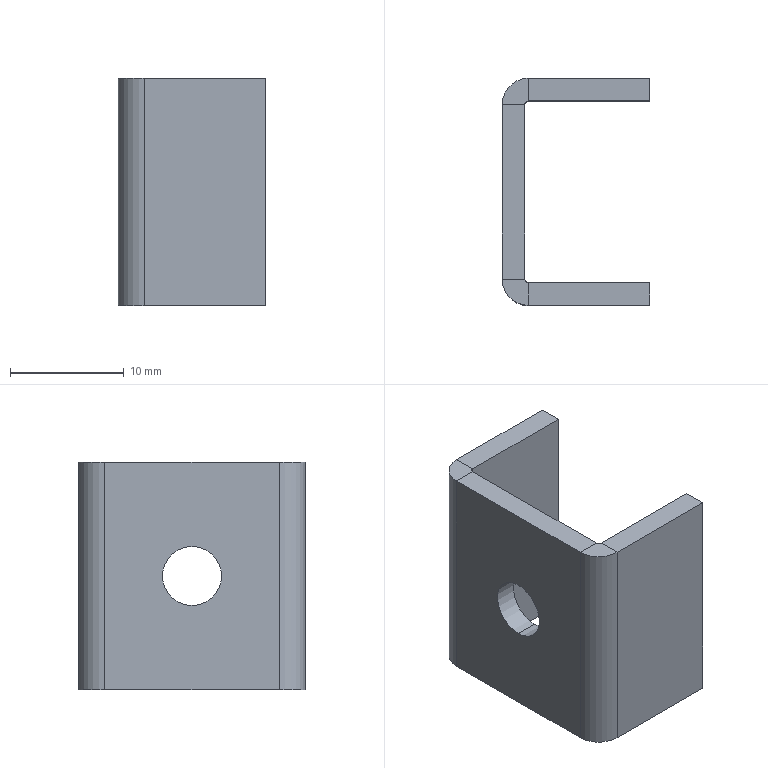Part | SolidWorks | features Cut 1, FlatPattern 1, SMBaseFlange 1, SheetMetal 1 | 1 solid | 24 faces | box 13 x 20 x 20 mm | volume 1593 mm3 | plane 18 | cylinder 6 | commonest cylinder face diameters 0.6 x2 4.6 x2 5.2 x2
STEP:
#1=CARTESIAN_POINT('',(2.,10.,7.4));
#2=VERTEX_POINT('',#1);
#3=CARTESIAN_POINT('',(2.,10.,12.6));
#4=VERTEX_POINT('',#3);
#5=CARTESIAN_POINT('',(2.,10.,10.));
#6=DIRECTION('',(-1.,0.,0.));
#7=DIRECTION('',(0.,0.,1.));
#8=AXIS2_PLACEMENT_3D('',#5,#6,#7);
#9=CIRCLE('',#8,2.6);
#10=EDGE_CURVE('',#2,#4,#9,.T.);
#11=ORIENTED_EDGE('',*,*,#10,.F.);
#12=CARTESIAN_POINT('',(0.,10.,7.4));
#13=VERTEX_POINT('',#12);
#14=CARTESIAN_POINT('',(2.,10.,7.4));
#15=DIRECTION('',(-1.,0.,0.));
#16=VECTOR('',#15,1000.);
#17=LINE('',#14,#16);
#18=EDGE_CURVE('',#2,#13,#17,.T.);
#19=ORIENTED_EDGE('',*,*,#18,.T.);
#20=CARTESIAN_POINT('',(0.,10.,12.6));
#21=VERTEX_POINT('',#20);
#22=CARTESIAN_POINT('',(0.,10.,10.));
#23=DIRECTION('',(-1.,0.,0.));
#24=DIRECTION('',(0.,0.,1.));
#25=AXIS2_PLACEMENT_3D('',#22,#23,#24);
#26=CIRCLE('',#25,2.6);
#27=EDGE_CURVE('',#13,#21,#26,.T.);
#28=ORIENTED_EDGE('',*,*,#27,.T.);
#29=CARTESIAN_POINT('',(2.,10.,12.6));
#30=DIRECTION('',(-1.,0.,0.));
#31=VECTOR('',#30,1000.);
#32=LINE('',#29,#31);
#33=EDGE_CURVE('',#4,#21,#32,.T.);
#34=ORIENTED_EDGE('',*,*,#33,.F.);
#35=EDGE_LOOP('',(#11,#19,#28,#34));
#36=FACE_OUTER_BOUND('',#35,.T.);
#37=CARTESIAN_POINT('',(2.,10.,10.));
#38=DIRECTION('',(-1.,0.,0.));
#39=DIRECTION('',(0.,0.,1.));
#40=AXIS2_PLACEMENT_3D('',#37,#38,#39);
#41=CYLINDRICAL_SURFACE('',#40,2.6);
#42=ADVANCED_FACE('',(#36),#41,.F.);
#43=CARTESIAN_POINT('',(0.,2.3,20.));
#44=VERTEX_POINT('',#43);
#45=CARTESIAN_POINT('',(2.,2.3,20.));
#46=VERTEX_POINT('',#45);
#47=CARTESIAN_POINT('',(0.,2.3,20.));
#48=DIRECTION('',(1.,0.,0.));
#49=VECTOR('',#48,1000.);
#50=LINE('',#47,#49);
#51=EDGE_CURVE('',#44,#46,#50,.T.);
#52=ORIENTED_EDGE('',*,*,#51,.F.);
#53=CARTESIAN_POINT('',(2.3,0.,20.));
#54=VERTEX_POINT('',#53);
#55=CARTESIAN_POINT('',(2.3,2.3,20.));
#56=DIRECTION('',(0.,0.,-1.));
#57=DIRECTION('',(1.,0.,0.));
#58=AXIS2_PLACEMENT_3D('',#55,#56,#57);
#59=CIRCLE('',#58,2.3);
#60=EDGE_CURVE('',#54,#44,#59,.T.);
#61=ORIENTED_EDGE('',*,*,#60,.F.);
#62=CARTESIAN_POINT('',(2.3,2.,20.));
#63=VERTEX_POINT('',#62);
#64=CARTESIAN_POINT('',(2.3,2.,20.));
#65=DIRECTION('',(0.,-1.,0.));
#66=VECTOR('',#65,1000.);
#67=LINE('',#64,#66);
#68=EDGE_CURVE('',#63,#54,#67,.T.);
#69=ORIENTED_EDGE('',*,*,#68,.F.);
#70=CARTESIAN_POINT('',(2.3,2.3,20.));
#71=DIRECTION('',(0.,0.,-1.));
#72=DIRECTION('',(1.,0.,0.));
#73=AXIS2_PLACEMENT_3D('',#70,#71,#72);
#74=CIRCLE('',#73,0.3);
#75=EDGE_CURVE('',#63,#46,#74,.T.);
#76=ORIENTED_EDGE('',*,*,#75,.T.);
#77=EDGE_LOOP('',(#52,#61,#69,#76));
#78=FACE_OUTER_BOUND('',#77,.T.);
#79=CARTESIAN_POINT('',(0.,2.3,20.));
#80=DIRECTION('',(0.,0.,1.));
#81=DIRECTION('',(1.,0.,0.));
#82=AXIS2_PLACEMENT_3D('',#79,#80,#81);
#83=PLANE('',#82);
#84=ADVANCED_FACE('',(#78),#83,.T.);
#85=CARTESIAN_POINT('',(0.,17.7,20.));
#86=VERTEX_POINT('',#85);
#87=CARTESIAN_POINT('',(0.,0.,20.));
#88=DIRECTION('',(0.,1.,0.));
#89=VECTOR('',#88,1000.);
#90=LINE('',#87,#89);
#91=EDGE_CURVE('',#44,#86,#90,.T.);
#92=ORIENTED_EDGE('',*,*,#91,.F.);
#93=ORIENTED_EDGE('',*,*,#51,.T.);
#94=CARTESIAN_POINT('',(2.,17.7,20.));
#95=VERTEX_POINT('',#94);
#96=CARTESIAN_POINT('',(2.,0.,20.));
#97=DIRECTION('',(0.,1.,0.));
#98=VECTOR('',#97,1000.);
#99=LINE('',#96,#98);
#100=EDGE_CURVE('',#46,#95,#99,.T.);
#101=ORIENTED_EDGE('',*,*,#100,.T.);
#102=CARTESIAN_POINT('',(2.,17.7,20.));
#103=DIRECTION('',(-1.,0.,0.));
#104=VECTOR('',#103,1000.);
#105=LINE('',#102,#104);
#106=EDGE_CURVE('',#95,#86,#105,.T.);
#107=ORIENTED_EDGE('',*,*,#106,.T.);
#108=EDGE_LOOP('',(#92,#93,#101,#107));
#109=FACE_OUTER_BOUND('',#108,.T.);
#110=CARTESIAN_POINT('',(2.3,2.,20.));
#111=DIRECTION('',(0.,0.,1.));
#112=DIRECTION('',(1.,0.,0.));
#113=AXIS2_PLACEMENT_3D('',#110,#111,#112);
#114=PLANE('',#113);
#115=ADVANCED_FACE('',(#109),#114,.T.);
#116=CARTESIAN_POINT('',(2.3,0.,0.));
#117=VERTEX_POINT('',#116);
#118=CARTESIAN_POINT('',(2.3,2.,0.));
#119=VERTEX_POINT('',#118);
#120=CARTESIAN_POINT('',(2.3,0.,0.));
#121=DIRECTION('',(0.,1.,0.));
#122=VECTOR('',#121,1000.);
#123=LINE('',#120,#122);
#124=EDGE_CURVE('',#117,#119,#123,.T.);
#125=ORIENTED_EDGE('',*,*,#124,.F.);
#126=CARTESIAN_POINT('',(0.,2.3,0.));
#127=VERTEX_POINT('',#126);
#128=CARTESIAN_POINT('',(2.3,2.3,0.));
#129=DIRECTION('',(0.,0.,-1.));
#130=DIRECTION('',(1.,0.,0.));
#131=AXIS2_PLACEMENT_3D('',#128,#129,#130);
#132=CIRCLE('',#131,2.3);
#133=EDGE_CURVE('',#117,#127,#132,.T.);
#134=ORIENTED_EDGE('',*,*,#133,.T.);
#135=CARTESIAN_POINT('',(2.,2.3,0.));
#136=VERTEX_POINT('',#135);
#137=CARTESIAN_POINT('',(2.,2.3,0.));
#138=DIRECTION('',(-1.,0.,0.));
#139=VECTOR('',#138,1000.);
#140=LINE('',#137,#139);
#141=EDGE_CURVE('',#136,#127,#140,.T.);
#142=ORIENTED_EDGE('',*,*,#141,.F.);
#143=CARTESIAN_POINT('',(2.3,2.3,0.));
#144=DIRECTION('',(0.,0.,-1.));
#145=DIRECTION('',(1.,0.,0.));
#146=AXIS2_PLACEMENT_3D('',#143,#144,#145);
#147=CIRCLE('',#146,0.3);
#148=EDGE_CURVE('',#119,#136,#147,.T.);
#149=ORIENTED_EDGE('',*,*,#148,.F.);
#150=EDGE_LOOP('',(#125,#134,#142,#149));
#151=FACE_OUTER_BOUND('',#150,.T.);
#152=CARTESIAN_POINT('',(2.3,0.,0.));
#153=DIRECTION('',(0.,0.,-1.));
#154=DIRECTION('',(-1.,0.,0.));
#155=AXIS2_PLACEMENT_3D('',#152,#153,#154);
#156=PLANE('',#155);
#157=ADVANCED_FACE('',(#151),#156,.T.);
#158=CARTESIAN_POINT('',(13.,0.,0.));
#159=VERTEX_POINT('',#158);
#160=CARTESIAN_POINT('',(13.,0.,0.));
#161=DIRECTION('',(-1.,0.,0.));
#162=VECTOR('',#161,1000.);
#163=LINE('',#160,#162);
#164=EDGE_CURVE('',#159,#117,#163,.T.);
#165=ORIENTED_EDGE('',*,*,#164,.T.);
#166=ORIENTED_EDGE('',*,*,#124,.T.);
#167=CARTESIAN_POINT('',(13.,2.,0.));
#168=VERTEX_POINT('',#167);
#169=CARTESIAN_POINT('',(13.,2.,0.));
#170=DIRECTION('',(-1.,0.,0.));
#171=VECTOR('',#170,1000.);
#172=LINE('',#169,#171);
#173=EDGE_CURVE('',#168,#119,#172,.T.);
#174=ORIENTED_EDGE('',*,*,#173,.F.);
#175=CARTESIAN_POINT('',(13.,2.,0.));
#176=DIRECTION('',(0.,-1.,0.));
#177=VECTOR('',#176,1000.);
#178=LINE('',#175,#177);
#179=EDGE_CURVE('',#168,#159,#178,.T.);
#180=ORIENTED_EDGE('',*,*,#179,.T.);
#181=EDGE_LOOP('',(#165,#166,#174,#180));
#182=FACE_OUTER_BOUND('',#181,.T.);
#183=CARTESIAN_POINT('',(2.,2.3,0.));
#184=DIRECTION('',(0.,0.,-1.));
#185=DIRECTION('',(-1.,0.,0.));
#186=AXIS2_PLACEMENT_3D('',#183,#184,#185);
#187=PLANE('',#186);
#188=ADVANCED_FACE('',(#182),#187,.T.);
#189=CARTESIAN_POINT('',(2.3,20.,20.));
#190=VERTEX_POINT('',#189);
#191=CARTESIAN_POINT('',(2.3,18.,20.));
#192=VERTEX_POINT('',#191);
#193=CARTESIAN_POINT('',(2.3,20.,20.));
#194=DIRECTION('',(0.,-1.,0.));
#195=VECTOR('',#194,1000.);
#196=LINE('',#193,#195);
#197=EDGE_CURVE('',#190,#192,#196,.T.);
#198=ORIENTED_EDGE('',*,*,#197,.F.);
#199=CARTESIAN_POINT('',(2.3,17.7,20.));
#200=DIRECTION('',(0.,0.,-1.));
#201=DIRECTION('',(1.,0.,0.));
#202=AXIS2_PLACEMENT_3D('',#199,#200,#201);
#203=CIRCLE('',#202,2.3);
#204=EDGE_CURVE('',#86,#190,#203,.T.);
#205=ORIENTED_EDGE('',*,*,#204,.F.);
#206=ORIENTED_EDGE('',*,*,#106,.F.);
#207=CARTESIAN_POINT('',(2.3,17.7,20.));
#208=DIRECTION('',(0.,0.,-1.));
#209=DIRECTION('',(1.,0.,0.));
#210=AXIS2_PLACEMENT_3D('',#207,#208,#209);
#211=CIRCLE('',#210,0.3);
#212=EDGE_CURVE('',#95,#192,#211,.T.);
#213=ORIENTED_EDGE('',*,*,#212,.T.);
#214=EDGE_LOOP('',(#198,#205,#206,#213));
#215=FACE_OUTER_BOUND('',#214,.T.);
#216=CARTESIAN_POINT('',(2.3,20.,20.));
#217=DIRECTION('',(0.,0.,1.));
#218=DIRECTION('',(1.,0.,0.));
#219=AXIS2_PLACEMENT_3D('',#216,#217,#218);
#220=PLANE('',#219);
#221=ADVANCED_FACE('',(#215),#220,.T.);
#222=CARTESIAN_POINT('',(13.,20.,20.));
#223=VERTEX_POINT('',#222);
#224=CARTESIAN_POINT('',(0.,20.,20.));
#225=DIRECTION('',(1.,0.,0.));
#226=VECTOR('',#225,1000.);
#227=LINE('',#224,#226);
#228=EDGE_CURVE('',#190,#223,#227,.T.);
#229=ORIENTED_EDGE('',*,*,#228,.F.);
#230=ORIENTED_EDGE('',*,*,#197,.T.);
#231=CARTESIAN_POINT('',(13.,18.,20.));
#232=VERTEX_POINT('',#231);
#233=CARTESIAN_POINT('',(0.,18.,20.));
#234=DIRECTION('',(1.,0.,0.));
#235=VECTOR('',#234,1000.);
#236=LINE('',#233,#235);
#237=EDGE_CURVE('',#192,#232,#236,.T.);
#238=ORIENTED_EDGE('',*,*,#237,.T.);
#239=CARTESIAN_POINT('',(13.,20.,20.));
#240=DIRECTION('',(0.,-1.,0.));
#241=VECTOR('',#240,1000.);
#242=LINE('',#239,#241);
#243=EDGE_CURVE('',#223,#232,#242,.T.);
#244=ORIENTED_EDGE('',*,*,#243,.F.);
#245=EDGE_LOOP('',(#229,#230,#238,#244));
#246=FACE_OUTER_BOUND('',#245,.T.);
#247=CARTESIAN_POINT('',(2.,17.7,20.));
#248=DIRECTION('',(0.,0.,1.));
#249=DIRECTION('',(1.,0.,0.));
#250=AXIS2_PLACEMENT_3D('',#247,#248,#249);
#251=PLANE('',#250);
#252=ADVANCED_FACE('',(#246),#251,.T.);
#253=CARTESIAN_POINT('',(0.,17.7,0.));
#254=VERTEX_POINT('',#253);
#255=CARTESIAN_POINT('',(2.,17.7,0.));
#256=VERTEX_POINT('',#255);
#257=CARTESIAN_POINT('',(0.,17.7,0.));
#258=DIRECTION('',(1.,0.,0.));
#259=VECTOR('',#258,1000.);
#260=LINE('',#257,#259);
#261=EDGE_CURVE('',#254,#256,#260,.T.);
#262=ORIENTED_EDGE('',*,*,#261,.F.);
#263=CARTESIAN_POINT('',(2.3,20.,0.));
#264=VERTEX_POINT('',#263);
#265=CARTESIAN_POINT('',(2.3,17.7,0.));
#266=DIRECTION('',(0.,0.,-1.));
#267=DIRECTION('',(1.,0.,0.));
#268=AXIS2_PLACEMENT_3D('',#265,#266,#267);
#269=CIRCLE('',#268,2.3);
#270=EDGE_CURVE('',#254,#264,#269,.T.);
#271=ORIENTED_EDGE('',*,*,#270,.T.);
#272=CARTESIAN_POINT('',(2.3,18.,0.));
#273=VERTEX_POINT('',#272);
#274=CARTESIAN_POINT('',(2.3,18.,0.));
#275=DIRECTION('',(0.,1.,0.));
#276=VECTOR('',#275,1000.);
#277=LINE('',#274,#276);
#278=EDGE_CURVE('',#273,#264,#277,.T.);
#279=ORIENTED_EDGE('',*,*,#278,.F.);
#280=CARTESIAN_POINT('',(2.3,17.7,0.));
#281=DIRECTION('',(0.,0.,-1.));
#282=DIRECTION('',(1.,0.,0.));
#283=AXIS2_PLACEMENT_3D('',#280,#281,#282);
#284=CIRCLE('',#283,0.3);
#285=EDGE_CURVE('',#256,#273,#284,.T.);
#286=ORIENTED_EDGE('',*,*,#285,.F.);
#287=EDGE_LOOP('',(#262,#271,#279,#286));
#288=FACE_OUTER_BOUND('',#287,.T.);
#289=CARTESIAN_POINT('',(0.,17.7,0.));
#290=DIRECTION('',(0.,0.,-1.));
#291=DIRECTION('',(-1.,0.,0.));
#292=AXIS2_PLACEMENT_3D('',#289,#290,#291);
#293=PLANE('',#292);
#294=ADVANCED_FACE('',(#288),#293,.T.);
#295=CARTESIAN_POINT('',(0.,0.,0.));
#296=DIRECTION('',(0.,1.,0.));
#297=VECTOR('',#296,1000.);
#298=LINE('',#295,#297);
#299=EDGE_CURVE('',#127,#254,#298,.T.);
#300=ORIENTED_EDGE('',*,*,#299,.T.);
#301=ORIENTED_EDGE('',*,*,#261,.T.);
#302=CARTESIAN_POINT('',(2.,0.,0.));
#303=DIRECTION('',(0.,1.,0.));
#304=VECTOR('',#303,1000.);
#305=LINE('',#302,#304);
#306=EDGE_CURVE('',#136,#256,#305,.T.);
#307=ORIENTED_EDGE('',*,*,#306,.F.);
#308=ORIENTED_EDGE('',*,*,#141,.T.);
#309=EDGE_LOOP('',(#300,#301,#307,#308));
#310=FACE_OUTER_BOUND('',#309,.T.);
#311=CARTESIAN_POINT('',(2.3,18.,0.));
#312=DIRECTION('',(0.,0.,-1.));
#313=DIRECTION('',(-1.,0.,0.));
#314=AXIS2_PLACEMENT_3D('',#311,#312,#313);
#315=PLANE('',#314);
#316=ADVANCED_FACE('',(#310),#315,.T.);
#317=CARTESIAN_POINT('',(13.,18.,0.));
#318=VERTEX_POINT('',#317);
#319=CARTESIAN_POINT('',(0.,18.,0.));
#320=DIRECTION('',(1.,0.,0.));
#321=VECTOR('',#320,1000.);
#322=LINE('',#319,#321);
#323=EDGE_CURVE('',#273,#318,#322,.T.);
#324=ORIENTED_EDGE('',*,*,#323,.T.);
#325=CARTESIAN_POINT('',(13.,18.,20.));
#326=DIRECTION('',(0.,0.,-1.));
#327=VECTOR('',#326,1000.);
#328=LINE('',#325,#327);
#329=EDGE_CURVE('',#232,#318,#328,.T.);
#330=ORIENTED_EDGE('',*,*,#329,.F.);
#331=ORIENTED_EDGE('',*,*,#237,.F.);
#332=CARTESIAN_POINT('',(2.3,18.,20.));
#333=DIRECTION('',(0.,0.,-1.));
#334=VECTOR('',#333,1000.);
#335=LINE('',#332,#334);
#336=EDGE_CURVE('',#192,#273,#335,.T.);
#337=ORIENTED_EDGE('',*,*,#336,.T.);
#338=EDGE_LOOP('',(#324,#330,#331,#337));
#339=FACE_OUTER_BOUND('',#338,.T.);
#340=CARTESIAN_POINT('',(0.,18.,20.));
#341=DIRECTION('',(0.,1.,0.));
#342=DIRECTION('',(0.,0.,1.));
#343=AXIS2_PLACEMENT_3D('',#340,#341,#342);
#344=PLANE('',#343);
#345=ADVANCED_FACE('',(#339),#344,.F.);
#346=CARTESIAN_POINT('',(13.,20.,0.));
#347=VERTEX_POINT('',#346);
#348=CARTESIAN_POINT('',(13.,20.,0.));
#349=DIRECTION('',(0.,-1.,0.));
#350=VECTOR('',#349,1000.);
#351=LINE('',#348,#350);
#352=EDGE_CURVE('',#347,#318,#351,.T.);
#353=ORIENTED_EDGE('',*,*,#352,.F.);
#354=CARTESIAN_POINT('',(13.,20.,20.));
#355=DIRECTION('',(0.,0.,-1.));
#356=VECTOR('',#355,1000.);
#357=LINE('',#354,#356);
#358=EDGE_CURVE('',#223,#347,#357,.T.);
#359=ORIENTED_EDGE('',*,*,#358,.F.);
#360=ORIENTED_EDGE('',*,*,#243,.T.);
#361=ORIENTED_EDGE('',*,*,#329,.T.);
#362=EDGE_LOOP('',(#353,#359,#360,#361));
#363=FACE_OUTER_BOUND('',#362,.T.);
#364=CARTESIAN_POINT('',(13.,20.,20.));
#365=DIRECTION('',(1.,0.,0.));
#366=DIRECTION('',(0.,0.,-1.));
#367=AXIS2_PLACEMENT_3D('',#364,#365,#366);
#368=PLANE('',#367);
#369=ADVANCED_FACE('',(#363),#368,.T.);
#370=CARTESIAN_POINT('',(0.,20.,0.));
#371=DIRECTION('',(1.,0.,0.));
#372=VECTOR('',#371,1000.);
#373=LINE('',#370,#372);
#374=EDGE_CURVE('',#264,#347,#373,.T.);
#375=ORIENTED_EDGE('',*,*,#374,.F.);
#376=CARTESIAN_POINT('',(2.3,20.,20.));
#377=DIRECTION('',(0.,0.,-1.));
#378=VECTOR('',#377,1000.);
#379=LINE('',#376,#378);
#380=EDGE_CURVE('',#190,#264,#379,.T.);
#381=ORIENTED_EDGE('',*,*,#380,.F.);
#382=ORIENTED_EDGE('',*,*,#228,.T.);
#383=ORIENTED_EDGE('',*,*,#358,.T.);
#384=EDGE_LOOP('',(#375,#381,#382,#383));
#385=FACE_OUTER_BOUND('',#384,.T.);
#386=CARTESIAN_POINT('',(0.,20.,20.));
#387=DIRECTION('',(0.,1.,0.));
#388=DIRECTION('',(0.,0.,1.));
#389=AXIS2_PLACEMENT_3D('',#386,#387,#388);
#390=PLANE('',#389);
#391=ADVANCED_FACE('',(#385),#390,.T.);
#392=ORIENTED_EDGE('',*,*,#270,.F.);
#393=CARTESIAN_POINT('',(0.,17.7,20.));
#394=DIRECTION('',(0.,0.,-1.));
#395=VECTOR('',#394,1000.);
#396=LINE('',#393,#395);
#397=EDGE_CURVE('',#86,#254,#396,.T.);
#398=ORIENTED_EDGE('',*,*,#397,.F.);
#399=ORIENTED_EDGE('',*,*,#204,.T.);
#400=ORIENTED_EDGE('',*,*,#380,.T.);
#401=EDGE_LOOP('',(#392,#398,#399,#400));
#402=FACE_OUTER_BOUND('',#401,.T.);
#403=CARTESIAN_POINT('',(2.3,17.7,20.));
#404=DIRECTION('',(0.,0.,-1.));
#405=DIRECTION('',(-1.,0.,0.));
#406=AXIS2_PLACEMENT_3D('',#403,#404,#405);
#407=CYLINDRICAL_SURFACE('',#406,2.3);
#408=ADVANCED_FACE('',(#402),#407,.T.);
#409=CARTESIAN_POINT('',(0.,10.,10.));
#410=DIRECTION('',(-1.,0.,0.));
#411=DIRECTION('',(0.,0.,1.));
#412=AXIS2_PLACEMENT_3D('',#409,#410,#411);
#413=CIRCLE('',#412,2.6);
#414=EDGE_CURVE('',#21,#13,#413,.T.);
#415=ORIENTED_EDGE('',*,*,#414,.F.);
#416=ORIENTED_EDGE('',*,*,#27,.F.);
#417=EDGE_LOOP('',(#415,#416));
#418=FACE_BOUND('',#417,.T.);
#419=ORIENTED_EDGE('',*,*,#299,.F.);
#420=CARTESIAN_POINT('',(0.,2.3,20.));
#421=DIRECTION('',(0.,0.,-1.));
#422=VECTOR('',#421,1000.);
#423=LINE('',#420,#422);
#424=EDGE_CURVE('',#44,#127,#423,.T.);
#425=ORIENTED_EDGE('',*,*,#424,.F.);
#426=ORIENTED_EDGE('',*,*,#91,.T.);
#427=ORIENTED_EDGE('',*,*,#397,.T.);
#428=EDGE_LOOP('',(#419,#425,#426,#427));
#429=FACE_OUTER_BOUND('',#428,.T.);
#430=CARTESIAN_POINT('',(0.,0.,20.));
#431=DIRECTION('',(-1.,0.,0.));
#432=DIRECTION('',(0.,0.,1.));
#433=AXIS2_PLACEMENT_3D('',#430,#431,#432);
#434=PLANE('',#433);
#435=ADVANCED_FACE('',(#418,#429),#434,.T.);
#436=ORIENTED_EDGE('',*,*,#133,.F.);
#437=CARTESIAN_POINT('',(2.3,0.,20.));
#438=DIRECTION('',(0.,0.,-1.));
#439=VECTOR('',#438,1000.);
#440=LINE('',#437,#439);
#441=EDGE_CURVE('',#54,#117,#440,.T.);
#442=ORIENTED_EDGE('',*,*,#441,.F.);
#443=ORIENTED_EDGE('',*,*,#60,.T.);
#444=ORIENTED_EDGE('',*,*,#424,.T.);
#445=EDGE_LOOP('',(#436,#442,#443,#444));
#446=FACE_OUTER_BOUND('',#445,.T.);
#447=CARTESIAN_POINT('',(2.3,2.3,20.));
#448=DIRECTION('',(0.,0.,-1.));
#449=DIRECTION('',(-1.,0.,0.));
#450=AXIS2_PLACEMENT_3D('',#447,#448,#449);
#451=CYLINDRICAL_SURFACE('',#450,2.3);
#452=ADVANCED_FACE('',(#446),#451,.T.);
#453=ORIENTED_EDGE('',*,*,#164,.F.);
#454=CARTESIAN_POINT('',(13.,0.,20.));
#455=VERTEX_POINT('',#454);
#456=CARTESIAN_POINT('',(13.,0.,20.));
#457=DIRECTION('',(0.,0.,-1.));
#458=VECTOR('',#457,1000.);
#459=LINE('',#456,#458);
#460=EDGE_CURVE('',#455,#159,#459,.T.);
#461=ORIENTED_EDGE('',*,*,#460,.F.);
#462=CARTESIAN_POINT('',(13.,0.,20.));
#463=DIRECTION('',(-1.,0.,0.));
#464=VECTOR('',#463,1000.);
#465=LINE('',#462,#464);
#466=EDGE_CURVE('',#455,#54,#465,.T.);
#467=ORIENTED_EDGE('',*,*,#466,.T.);
#468=ORIENTED_EDGE('',*,*,#441,.T.);
#469=EDGE_LOOP('',(#453,#461,#467,#468));
#470=FACE_OUTER_BOUND('',#469,.T.);
#471=CARTESIAN_POINT('',(13.,0.,20.));
#472=DIRECTION('',(0.,-1.,0.));
#473=DIRECTION('',(1.,0.,0.));
#474=AXIS2_PLACEMENT_3D('',#471,#472,#473);
#475=PLANE('',#474);
#476=ADVANCED_FACE('',(#470),#475,.T.);
#477=ORIENTED_EDGE('',*,*,#179,.F.);
#478=CARTESIAN_POINT('',(13.,2.,20.));
#479=VERTEX_POINT('',#478);
#480=CARTESIAN_POINT('',(13.,2.,20.));
#481=DIRECTION('',(0.,0.,-1.));
#482=VECTOR('',#481,1000.);
#483=LINE('',#480,#482);
#484=EDGE_CURVE('',#479,#168,#483,.T.);
#485=ORIENTED_EDGE('',*,*,#484,.F.);
#486=CARTESIAN_POINT('',(13.,2.,20.));
#487=DIRECTION('',(0.,-1.,0.));
#488=VECTOR('',#487,1000.);
#489=LINE('',#486,#488);
#490=EDGE_CURVE('',#479,#455,#489,.T.);
#491=ORIENTED_EDGE('',*,*,#490,.T.);
#492=ORIENTED_EDGE('',*,*,#460,.T.);
#493=EDGE_LOOP('',(#477,#485,#491,#492));
#494=FACE_OUTER_BOUND('',#493,.T.);
#495=CARTESIAN_POINT('',(13.,2.,20.));
#496=DIRECTION('',(1.,0.,0.));
#497=DIRECTION('',(0.,0.,-1.));
#498=AXIS2_PLACEMENT_3D('',#495,#496,#497);
#499=PLANE('',#498);
#500=ADVANCED_FACE('',(#494),#499,.T.);
#501=ORIENTED_EDGE('',*,*,#173,.T.);
#502=CARTESIAN_POINT('',(2.3,2.,20.));
#503=DIRECTION('',(0.,0.,-1.));
#504=VECTOR('',#503,1000.);
#505=LINE('',#502,#504);
#506=EDGE_CURVE('',#63,#119,#505,.T.);
#507=ORIENTED_EDGE('',*,*,#506,.F.);
#508=CARTESIAN_POINT('',(13.,2.,20.));
#509=DIRECTION('',(-1.,0.,0.));
#510=VECTOR('',#509,1000.);
#511=LINE('',#508,#510);
#512=EDGE_CURVE('',#479,#63,#511,.T.);
#513=ORIENTED_EDGE('',*,*,#512,.F.);
#514=ORIENTED_EDGE('',*,*,#484,.T.);
#515=EDGE_LOOP('',(#501,#507,#513,#514));
#516=FACE_OUTER_BOUND('',#515,.T.);
#517=CARTESIAN_POINT('',(13.,2.,20.));
#518=DIRECTION('',(0.,-1.,0.));
#519=DIRECTION('',(1.,0.,0.));
#520=AXIS2_PLACEMENT_3D('',#517,#518,#519);
#521=PLANE('',#520);
#522=ADVANCED_FACE('',(#516),#521,.F.);
#523=ORIENTED_EDGE('',*,*,#148,.T.);
#524=CARTESIAN_POINT('',(2.,2.3,20.));
#525=DIRECTION('',(0.,0.,-1.));
#526=VECTOR('',#525,1000.);
#527=LINE('',#524,#526);
#528=EDGE_CURVE('',#46,#136,#527,.T.);
#529=ORIENTED_EDGE('',*,*,#528,.F.);
#530=ORIENTED_EDGE('',*,*,#75,.F.);
#531=ORIENTED_EDGE('',*,*,#506,.T.);
#532=EDGE_LOOP('',(#523,#529,#530,#531));
#533=FACE_OUTER_BOUND('',#532,.T.);
#534=CARTESIAN_POINT('',(2.3,2.3,20.));
#535=DIRECTION('',(0.,0.,-1.));
#536=DIRECTION('',(-1.,0.,0.));
#537=AXIS2_PLACEMENT_3D('',#534,#535,#536);
#538=CYLINDRICAL_SURFACE('',#537,0.3);
#539=ADVANCED_FACE('',(#533),#538,.F.);
#540=CARTESIAN_POINT('',(2.,10.,10.));
#541=DIRECTION('',(-1.,0.,0.));
#542=DIRECTION('',(0.,0.,1.));
#543=AXIS2_PLACEMENT_3D('',#540,#541,#542);
#544=CIRCLE('',#543,2.6);
#545=EDGE_CURVE('',#4,#2,#544,.T.);
#546=ORIENTED_EDGE('',*,*,#545,.T.);
#547=ORIENTED_EDGE('',*,*,#10,.T.);
#548=EDGE_LOOP('',(#546,#547));
#549=FACE_BOUND('',#548,.T.);
#550=ORIENTED_EDGE('',*,*,#306,.T.);
#551=CARTESIAN_POINT('',(2.,17.7,20.));
#552=DIRECTION('',(0.,0.,-1.));
#553=VECTOR('',#552,1000.);
#554=LINE('',#551,#553);
#555=EDGE_CURVE('',#95,#256,#554,.T.);
#556=ORIENTED_EDGE('',*,*,#555,.F.);
#557=ORIENTED_EDGE('',*,*,#100,.F.);
#558=ORIENTED_EDGE('',*,*,#528,.T.);
#559=EDGE_LOOP('',(#550,#556,#557,#558));
#560=FACE_OUTER_BOUND('',#559,.T.);
#561=CARTESIAN_POINT('',(2.,0.,20.));
#562=DIRECTION('',(-1.,0.,0.));
#563=DIRECTION('',(0.,0.,1.));
#564=AXIS2_PLACEMENT_3D('',#561,#562,#563);
#565=PLANE('',#564);
#566=ADVANCED_FACE('',(#549,#560),#565,.F.);
#567=ORIENTED_EDGE('',*,*,#285,.T.);
#568=ORIENTED_EDGE('',*,*,#336,.F.);
#569=ORIENTED_EDGE('',*,*,#212,.F.);
#570=ORIENTED_EDGE('',*,*,#555,.T.);
#571=EDGE_LOOP('',(#567,#568,#569,#570));
#572=FACE_OUTER_BOUND('',#571,.T.);
#573=CARTESIAN_POINT('',(2.3,17.7,20.));
#574=DIRECTION('',(0.,0.,-1.));
#575=DIRECTION('',(-1.,0.,0.));
#576=AXIS2_PLACEMENT_3D('',#573,#574,#575);
#577=CYLINDRICAL_SURFACE('',#576,0.3);
#578=ADVANCED_FACE('',(#572),#577,.F.);
#579=ORIENTED_EDGE('',*,*,#512,.T.);
#580=ORIENTED_EDGE('',*,*,#68,.T.);
#581=ORIENTED_EDGE('',*,*,#466,.F.);
#582=ORIENTED_EDGE('',*,*,#490,.F.);
#583=EDGE_LOOP('',(#579,#580,#581,#582));
#584=FACE_OUTER_BOUND('',#583,.T.);
#585=CARTESIAN_POINT('',(2.3,17.7,20.));
#586=DIRECTION('',(0.,0.,1.));
#587=DIRECTION('',(1.,0.,0.));
#588=AXIS2_PLACEMENT_3D('',#585,#586,#587);
#589=PLANE('',#588);
#590=ADVANCED_FACE('',(#584),#589,.T.);
#591=ORIENTED_EDGE('',*,*,#323,.F.);
#592=ORIENTED_EDGE('',*,*,#278,.T.);
#593=ORIENTED_EDGE('',*,*,#374,.T.);
#594=ORIENTED_EDGE('',*,*,#352,.T.);
#595=EDGE_LOOP('',(#591,#592,#593,#594));
#596=FACE_OUTER_BOUND('',#595,.T.);
#597=CARTESIAN_POINT('',(2.3,17.7,0.));
#598=DIRECTION('',(0.,0.,1.));
#599=DIRECTION('',(1.,0.,0.));
#600=AXIS2_PLACEMENT_3D('',#597,#598,#599);
#601=PLANE('',#600);
#602=ADVANCED_FACE('',(#596),#601,.F.);
#603=ORIENTED_EDGE('',*,*,#18,.F.);
#604=ORIENTED_EDGE('',*,*,#545,.F.);
#605=ORIENTED_EDGE('',*,*,#33,.T.);
#606=ORIENTED_EDGE('',*,*,#414,.T.);
#607=EDGE_LOOP('',(#603,#604,#605,#606));
#608=FACE_OUTER_BOUND('',#607,.T.);
#609=CARTESIAN_POINT('',(2.,10.,10.));
#610=DIRECTION('',(-1.,0.,0.));
#611=DIRECTION('',(0.,0.,1.));
#612=AXIS2_PLACEMENT_3D('',#609,#610,#611);
#613=CYLINDRICAL_SURFACE('',#612,2.6);
#614=ADVANCED_FACE('',(#608),#613,.F.);
#615=CLOSED_SHELL('',(#42,#84,#115,#157,#188,#221,#252,#294,#316,#345,#369,#391,#408,#435,#452,#476,#500,#522,#539,#566,#578,#590,#602,#614));
#616=MANIFOLD_SOLID_BREP('',#615);
#617=CARTESIAN_POINT('',(0.,0.,0.));
#618=DIRECTION('',(0.,0.,1.));
#619=DIRECTION('',(1.,0.,0.));
#620=AXIS2_PLACEMENT_3D('',#617,#618,#619);
#621=(LENGTH_UNIT()NAMED_UNIT(*)SI_UNIT(.MILLI.,.METRE.));
#622=UNCERTAINTY_MEASURE_WITH_UNIT(LENGTH_MEASURE(0.00001),#621,'','');
#623=(NAMED_UNIT(*)PLANE_ANGLE_UNIT()SI_UNIT($,.RADIAN.));
#624=(NAMED_UNIT(*)SI_UNIT($,.STERADIAN.)SOLID_ANGLE_UNIT());
#625=(GEOMETRIC_REPRESENTATION_CONTEXT(3)GLOBAL_UNCERTAINTY_ASSIGNED_CONTEXT((#622))GLOBAL_UNIT_ASSIGNED_CONTEXT((#621,#623,#624))REPRESENTATION_CONTEXT('',''));
#626=ADVANCED_BREP_SHAPE_REPRESENTATION('',(#616,#620),#625);